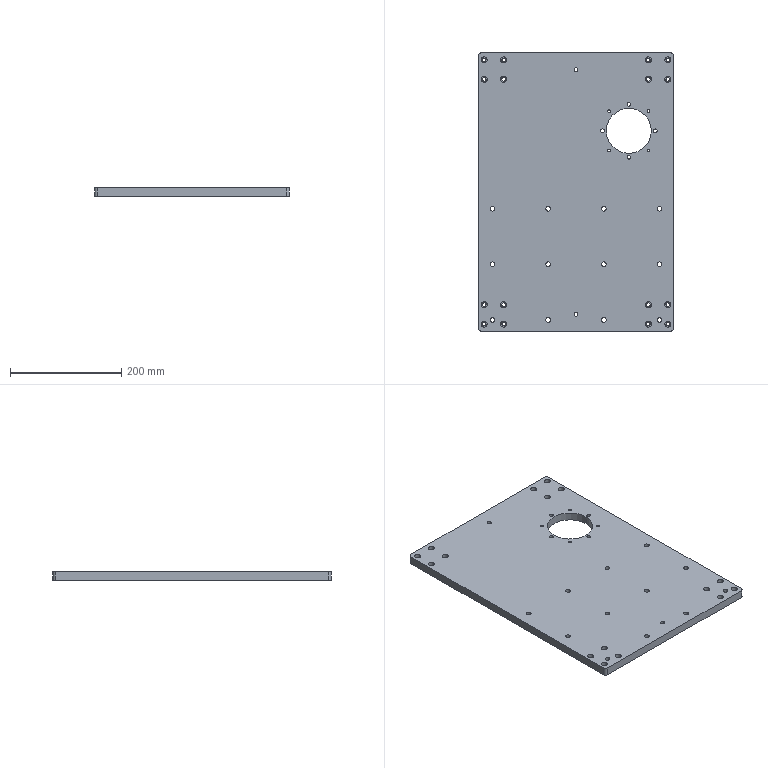NC program | Mastercam | posted with a generic post | part box 350 x 500 x 15 mm
Lines 1 to 1450 of 4195:
%
O0000()
(MATERIAL - ALUMINUM MM - 2024)
( T24 | 100 FEM | H24 )
( T9 | 10 FEM | H9 | XY STOCK TO LEAVE - .15 | Z STOCK TO LEAVE - .05 )
( T10 | 10 FEM | H10 | XY STOCK TO LEAVE - 0. | Z STOCK TO LEAVE - .05 )
( T7 | 4 CHM | H7 )
( T6 | 6 FEM | H6 )
N100 G21
N110 G0 G17 G40 G49 G80 G90
N120 T24 M6
N130 G0 G90 G54 X-360. Y144.998 A0. S4000 M3
N140 G43 H24 Z50. M8
N150 Z2.
N160 G1 Z0. F600.
N170 X300. F1000.
N180 G2 X336.249 Y108.749 I0. J-36.249
N190 X300. Y72.499 I-36.249 J0.
N200 G1 X-300.
N210 G3 X-336.25 Y36.249 I0. J-36.25
N220 X-300. Y0. I36.25 J0.
N230 G1 X300.
N240 G2 X336.249 Y-36.249 I0. J-36.249
N250 X300. Y-72.499 I-36.249 J0.
N260 G1 X-300.
N270 G3 X-336.25 Y-108.749 I0. J-36.25
N280 X-300. Y-144.998 I36.25 J0.
N290 G1 X360.
N300 G0 Z50.
N310 M5
N320 G91 G28 Z0. M9
N330 A0.
N340 M01
N350 T9 M6
N360 G0 G90 G17 G54 X-257.127 Y180.713 A0. S7000 M3
N370 G43 H9 Z50. M8
N380 Z1.
N390 G1 Z0. F600.
N400 X-253.591 Y177.177 F3000.
N410 G3 X-252.884 Y176.884 I.707 J.707
N420 X-252.177 Y177.177 I0. J1.
N430 G1 X-251.592 Y177.718
N440 X-250.966 Y178.211
N450 X-250.303 Y178.654 Z-.001
N460 X-249.608 Y179.044
N470 X-248.884 Y179.377
N480 X-248.136 Y179.653
N490 X-247.369 Y179.869
N500 X-246.588 Y180.025 Z-.002
N510 X-245.796 Y180.119
N520 X-245. Y180.15
N530 X245. Z-.144
N540 G2 X255.15 Y170. Z-.149 I0. J-10.15
N550 G1 Y-170. Z-.248
N560 X255.115 Y-170.838
N570 X255.012 Y-171.671
N580 X254.839 Y-172.492 Z-.249
N590 X254.6 Y-173.296
N600 X254.295 Y-174.077
N610 X253.927 Y-174.831
N620 X253.497 Y-175.552
N630 X253.01 Y-176.234 Z-.25
N640 X252.468 Y-176.874
N650 X251.874 Y-177.468
N660 X251.234 Y-178.01
N670 X250.552 Y-178.497 Z-.251
N680 X249.831 Y-178.927
N690 X249.077 Y-179.295
N700 X248.296 Y-179.6
N710 X247.492 Y-179.839
N720 X246.671 Y-180.012 Z-.252
N730 X245.838 Y-180.115
N740 X245. Y-180.15
N750 X-245. Z-.394
N760 G2 X-255.15 Y-170. Z-.399 I0. J10.15
N770 G1 Y170. Z-.498
N780 X-255.119 Y170.796
N790 X-255.025 Y171.588
N800 X-254.87 Y172.369 Z-.499
N810 X-254.653 Y173.137
N820 X-254.377 Y173.884
N830 X-254.044 Y174.608
N840 X-253.654 Y175.303
N850 X-253.212 Y175.966 Z-.5
N860 X-252.718 Y176.592
N870 X-252.177 Y177.177
N880 X-251.592 Y177.718
N890 X-250.966 Y178.211
N900 X-250.303 Y178.654 Z-.501
N910 X-249.608 Y179.044
N920 X-248.884 Y179.377
N930 X-248.136 Y179.653
N940 X-247.369 Y179.869
N950 X-246.588 Y180.025 Z-.502
N960 X-245.796 Y180.119
N970 X-245. Y180.15
N980 X245. Z-.644
N990 G2 X255.15 Y170. Z-.649 I0. J-10.15
N1000 G1 Y-170. Z-.748
N1010 X255.115 Y-170.838
N1020 X255.012 Y-171.671
N1030 X254.839 Y-172.492 Z-.749
N1040 X254.6 Y-173.296
N1050 X254.295 Y-174.077
N1060 X253.927 Y-174.831
N1070 X253.497 Y-175.552
N1080 X253.01 Y-176.234 Z-.75
N1090 X252.468 Y-176.874
N1100 X251.874 Y-177.468
N1110 X251.234 Y-178.01
N1120 X250.552 Y-178.497 Z-.751
N1130 X249.831 Y-178.927
N1140 X249.077 Y-179.295
N1150 X248.296 Y-179.6
N1160 X247.492 Y-179.839
N1170 X246.671 Y-180.012 Z-.752
N1180 X245.838 Y-180.115
N1190 X245. Y-180.15
N1200 X-245. Z-.894
N1210 G2 X-255.15 Y-170. Z-.899 I0. J10.15
N1220 G1 Y170. Z-.998
N1230 X-255.119 Y170.796
N1240 X-255.025 Y171.588
N1250 X-254.87 Y172.369 Z-.999
N1260 X-254.653 Y173.137
N1270 X-254.377 Y173.884
N1280 X-254.044 Y174.608
N1290 X-253.654 Y175.303
N1300 X-253.212 Y175.966 Z-1.
N1310 X-252.718 Y176.592
N1320 X-252.177 Y177.177
N1330 X-251.592 Y177.718
N1340 X-250.966 Y178.211
N1350 X-250.303 Y178.654 Z-1.001
N1360 X-249.608 Y179.044
N1370 X-248.884 Y179.377
N1380 X-248.136 Y179.653
N1390 X-247.369 Y179.869
N1400 X-246.588 Y180.025 Z-1.002
N1410 X-245.796 Y180.119
N1420 X-245. Y180.15
N1430 X245. Z-1.144
N1440 G2 X255.15 Y170. Z-1.149 I0. J-10.15
N1450 G1 Y-170. Z-1.248
N1460 X255.115 Y-170.838
N1470 X255.012 Y-171.671
N1480 X254.839 Y-172.492 Z-1.249
N1490 X254.6 Y-173.296
N1500 X254.295 Y-174.077
N1510 X253.927 Y-174.831
N1520 X253.497 Y-175.552
N1530 X253.01 Y-176.234 Z-1.25
N1540 X252.468 Y-176.874
N1550 X251.874 Y-177.468
N1560 X251.234 Y-178.01
N1570 X250.552 Y-178.497 Z-1.251
N1580 X249.831 Y-178.927
N1590 X249.077 Y-179.295
N1600 X248.296 Y-179.6
N1610 X247.492 Y-179.839
N1620 X246.671 Y-180.012 Z-1.252
N1630 X245.838 Y-180.115
N1640 X245. Y-180.15
N1650 X-245. Z-1.394
N1660 G2 X-255.15 Y-170. Z-1.399 I0. J10.15
N1670 G1 Y170. Z-1.498
N1680 X-255.119 Y170.796
N1690 X-255.025 Y171.588
N1700 X-254.87 Y172.369 Z-1.499
N1710 X-254.653 Y173.137
N1720 X-254.377 Y173.884
N1730 X-254.044 Y174.608
N1740 X-253.654 Y175.303
N1750 X-253.212 Y175.966 Z-1.5
N1760 X-252.718 Y176.592
N1770 X-252.177 Y177.177
N1780 X-251.592 Y177.718
N1790 X-250.966 Y178.211
N1800 X-250.303 Y178.654 Z-1.501
N1810 X-249.608 Y179.044
N1820 X-248.884 Y179.377
N1830 X-248.136 Y179.653
N1840 X-247.369 Y179.869
N1850 X-246.588 Y180.025 Z-1.502
N1860 X-245.796 Y180.119
N1870 X-245. Y180.15
N1880 X245. Z-1.644
N1890 G2 X255.15 Y170. Z-1.649 I0. J-10.15
N1900 G1 Y-170. Z-1.748
N1910 X255.115 Y-170.838
N1920 X255.012 Y-171.671
N1930 X254.839 Y-172.492 Z-1.749
N1940 X254.6 Y-173.296
N1950 X254.295 Y-174.077
N1960 X253.927 Y-174.831
N1970 X253.497 Y-175.552
N1980 X253.01 Y-176.234 Z-1.75
N1990 X252.468 Y-176.874
N2000 X251.874 Y-177.468
N2010 X251.234 Y-178.01
N2020 X250.552 Y-178.497 Z-1.751
N2030 X249.831 Y-178.927
N2040 X249.077 Y-179.295
N2050 X248.296 Y-179.6
N2060 X247.492 Y-179.839
N2070 X246.671 Y-180.012 Z-1.752
N2080 X245.838 Y-180.115
N2090 X245. Y-180.15
N2100 X-245. Z-1.894
N2110 G2 X-255.15 Y-170. Z-1.899 I0. J10.15
N2120 G1 Y170. Z-1.998
N2130 X-255.119 Y170.796
N2140 X-255.025 Y171.588
N2150 X-254.87 Y172.369 Z-1.999
N2160 X-254.653 Y173.137
N2170 X-254.377 Y173.884
N2180 X-254.044 Y174.608
N2190 X-253.654 Y175.303
N2200 X-253.212 Y175.966 Z-2.
N2210 X-252.718 Y176.592
N2220 X-252.177 Y177.177
N2230 X-251.592 Y177.718
N2240 X-250.966 Y178.211
N2250 X-250.303 Y178.654 Z-2.001
N2260 X-249.608 Y179.044
N2270 X-248.884 Y179.377
N2280 X-248.136 Y179.653
N2290 X-247.369 Y179.869
N2300 X-246.588 Y180.025 Z-2.002
N2310 X-245.796 Y180.119
N2320 X-245. Y180.15
N2330 X245. Z-2.144
N2340 G2 X255.15 Y170. Z-2.149 I0. J-10.15
N2350 G1 Y-170. Z-2.248
N2360 X255.115 Y-170.838
N2370 X255.012 Y-171.671
N2380 X254.839 Y-172.492 Z-2.249
N2390 X254.6 Y-173.296
N2400 X254.295 Y-174.077
N2410 X253.927 Y-174.831
N2420 X253.497 Y-175.552
N2430 X253.01 Y-176.234 Z-2.25
N2440 X252.468 Y-176.874
N2450 X251.874 Y-177.468
N2460 X251.234 Y-178.01
N2470 X250.552 Y-178.497 Z-2.251
N2480 X249.831 Y-178.927
N2490 X249.077 Y-179.295
N2500 X248.296 Y-179.6
N2510 X247.492 Y-179.839
N2520 X246.671 Y-180.012 Z-2.252
N2530 X245.838 Y-180.115
N2540 X245. Y-180.15
N2550 X-245. Z-2.394
N2560 G2 X-255.15 Y-170. Z-2.399 I0. J10.15
N2570 G1 Y170. Z-2.498
N2580 X-255.119 Y170.796
N2590 X-255.025 Y171.588
N2600 X-254.87 Y172.369 Z-2.499
N2610 X-254.653 Y173.137
N2620 X-254.377 Y173.884
N2630 X-254.044 Y174.608
N2640 X-253.654 Y175.303
N2650 X-253.212 Y175.966 Z-2.5
N2660 X-252.718 Y176.592
N2670 X-252.177 Y177.177
N2680 X-251.592 Y177.718
N2690 X-250.966 Y178.211
N2700 X-250.303 Y178.654 Z-2.501
N2710 X-249.608 Y179.044
N2720 X-248.884 Y179.377
N2730 X-248.136 Y179.653
N2740 X-247.369 Y179.869
N2750 X-246.588 Y180.025 Z-2.502
N2760 X-245.796 Y180.119
N2770 X-245. Y180.15
N2780 X245. Z-2.644
N2790 G2 X255.15 Y170. Z-2.649 I0. J-10.15
N2800 G1 Y-170. Z-2.748
N2810 X255.115 Y-170.838
N2820 X255.012 Y-171.671
N2830 X254.839 Y-172.492 Z-2.749
N2840 X254.6 Y-173.296
N2850 X254.295 Y-174.077
N2860 X253.927 Y-174.831
N2870 X253.497 Y-175.552
N2880 X253.01 Y-176.234 Z-2.75
N2890 X252.468 Y-176.874
N2900 X251.874 Y-177.468
N2910 X251.234 Y-178.01
N2920 X250.552 Y-178.497 Z-2.751
N2930 X249.831 Y-178.927
N2940 X249.077 Y-179.295
N2950 X248.296 Y-179.6
N2960 X247.492 Y-179.839
N2970 X246.671 Y-180.012 Z-2.752
N2980 X245.838 Y-180.115
N2990 X245. Y-180.15
N3000 X-245. Z-2.894
N3010 G2 X-255.15 Y-170. Z-2.899 I0. J10.15
N3020 G1 Y170. Z-2.998
N3030 X-255.119 Y170.796
N3040 X-255.025 Y171.588
N3050 X-254.87 Y172.369 Z-2.999
N3060 X-254.653 Y173.137
N3070 X-254.377 Y173.884
N3080 X-254.044 Y174.608
N3090 X-253.654 Y175.303
N3100 X-253.212 Y175.966 Z-3.
N3110 X-252.718 Y176.592
N3120 X-252.177 Y177.177
N3130 X-251.592 Y177.718
N3140 X-250.966 Y178.211
N3150 X-250.303 Y178.654 Z-3.001
N3160 X-249.608 Y179.044
N3170 X-248.884 Y179.377
N3180 X-248.136 Y179.653
N3190 X-247.369 Y179.869
N3200 X-246.588 Y180.025 Z-3.002
N3210 X-245.796 Y180.119
N3220 X-245. Y180.15
N3230 X245. Z-3.144
N3240 G2 X255.15 Y170. Z-3.149 I0. J-10.15
N3250 G1 Y-170. Z-3.248
N3260 X255.115 Y-170.838
N3270 X255.012 Y-171.671
N3280 X254.839 Y-172.492 Z-3.249
N3290 X254.6 Y-173.296
N3300 X254.295 Y-174.077
N3310 X253.927 Y-174.831
N3320 X253.497 Y-175.552
N3330 X253.01 Y-176.234 Z-3.25
N3340 X252.468 Y-176.874
N3350 X251.874 Y-177.468
N3360 X251.234 Y-178.01
N3370 X250.552 Y-178.497 Z-3.251
N3380 X249.831 Y-178.927
N3390 X249.077 Y-179.295
N3400 X248.296 Y-179.6
N3410 X247.492 Y-179.839
N3420 X246.671 Y-180.012 Z-3.252
N3430 X245.838 Y-180.115
N3440 X245. Y-180.15
N3450 X-245. Z-3.394
N3460 G2 X-255.15 Y-170. Z-3.399 I0. J10.15
N3470 G1 Y170. Z-3.498
N3480 X-255.119 Y170.796
N3490 X-255.025 Y171.588
N3500 X-254.87 Y172.369 Z-3.499
N3510 X-254.653 Y173.137
N3520 X-254.377 Y173.884
N3530 X-254.044 Y174.608
N3540 X-253.654 Y175.303
N3550 X-253.212 Y175.966 Z-3.5
N3560 X-252.718 Y176.592
N3570 X-252.177 Y177.177
N3580 X-251.592 Y177.718
N3590 X-250.966 Y178.211
N3600 X-250.303 Y178.654 Z-3.501
N3610 X-249.608 Y179.044
N3620 X-248.884 Y179.377
N3630 X-248.136 Y179.653
N3640 X-247.369 Y179.869
N3650 X-246.588 Y180.025 Z-3.502
N3660 X-245.796 Y180.119
N3670 X-245. Y180.15
N3680 X245. Z-3.644
N3690 G2 X255.15 Y170. Z-3.649 I0. J-10.15
N3700 G1 Y-170. Z-3.748
N3710 X255.115 Y-170.838
N3720 X255.012 Y-171.671
N3730 X254.839 Y-172.492 Z-3.749
N3740 X254.6 Y-173.296
N3750 X254.295 Y-174.077
N3760 X253.927 Y-174.831
N3770 X253.497 Y-175.552
N3780 X253.01 Y-176.234 Z-3.75
N3790 X252.468 Y-176.874
N3800 X251.874 Y-177.468
N3810 X251.234 Y-178.01
N3820 X250.552 Y-178.497 Z-3.751
N3830 X249.831 Y-178.927
N3840 X249.077 Y-179.295
N3850 X248.296 Y-179.6
N3860 X247.492 Y-179.839
N3870 X246.671 Y-180.012 Z-3.752
N3880 X245.838 Y-180.115
N3890 X245. Y-180.15
N3900 X-245. Z-3.894
N3910 G2 X-255.15 Y-170. Z-3.899 I0. J10.15
N3920 G1 Y170. Z-3.998
N3930 X-255.119 Y170.796
N3940 X-255.025 Y171.588
N3950 X-254.87 Y172.369 Z-3.999
N3960 X-254.653 Y173.137
N3970 X-254.377 Y173.884
N3980 X-254.044 Y174.608
N3990 X-253.654 Y175.303
N4000 X-253.212 Y175.966 Z-4.
N4010 X-252.718 Y176.592
N4020 X-252.177 Y177.177
N4030 X-251.592 Y177.718
N4040 X-250.966 Y178.211
N4050 X-250.303 Y178.654 Z-4.001
N4060 X-249.608 Y179.044
N4070 X-248.884 Y179.377
N4080 X-248.136 Y179.653
N4090 X-247.369 Y179.869
N4100 X-246.588 Y180.025 Z-4.002
N4110 X-245.796 Y180.119
N4120 X-245. Y180.15
N4130 X245. Z-4.144
N4140 G2 X255.15 Y170. Z-4.149 I0. J-10.15
N4150 G1 Y-170. Z-4.248
N4160 X255.115 Y-170.838
N4170 X255.012 Y-171.671
N4180 X254.839 Y-172.492 Z-4.249
N4190 X254.6 Y-173.296
N4200 X254.295 Y-174.077
N4210 X253.927 Y-174.831
N4220 X253.497 Y-175.552
N4230 X253.01 Y-176.234 Z-4.25
N4240 X252.468 Y-176.874
N4250 X251.874 Y-177.468
N4260 X251.234 Y-178.01
N4270 X250.552 Y-178.497 Z-4.251
N4280 X249.831 Y-178.927
N4290 X249.077 Y-179.295
N4300 X248.296 Y-179.6
N4310 X247.492 Y-179.839
N4320 X246.671 Y-180.012 Z-4.252
N4330 X245.838 Y-180.115
N4340 X245. Y-180.15
N4350 X-245. Z-4.394
N4360 G2 X-255.15 Y-170. Z-4.399 I0. J10.15
N4370 G1 Y170. Z-4.498
N4380 X-255.119 Y170.796
N4390 X-255.025 Y171.588
N4400 X-254.87 Y172.369 Z-4.499
N4410 X-254.653 Y173.137
N4420 X-254.377 Y173.884
N4430 X-254.044 Y174.608
N4440 X-253.654 Y175.303
N4450 X-253.212 Y175.966 Z-4.5
N4460 X-252.718 Y176.592
N4470 X-252.177 Y177.177
N4480 X-251.592 Y177.718
N4490 X-250.966 Y178.211
N4500 X-250.303 Y178.654 Z-4.501
N4510 X-249.608 Y179.044
N4520 X-248.884 Y179.377
N4530 X-248.136 Y179.653
N4540 X-247.369 Y179.869
N4550 X-246.588 Y180.025 Z-4.502
N4560 X-245.796 Y180.119
N4570 X-245. Y180.15
N4580 X245. Z-4.644
N4590 G2 X255.15 Y170. Z-4.649 I0. J-10.15
N4600 G1 Y-170. Z-4.748
N4610 X255.115 Y-170.838
N4620 X255.012 Y-171.671
N4630 X254.839 Y-172.492 Z-4.749
N4640 X254.6 Y-173.296
N4650 X254.295 Y-174.077
N4660 X253.927 Y-174.831
N4670 X253.497 Y-175.552
N4680 X253.01 Y-176.234 Z-4.75
N4690 X252.468 Y-176.874
N4700 X251.874 Y-177.468
N4710 X251.234 Y-178.01
N4720 X250.552 Y-178.497 Z-4.751
N4730 X249.831 Y-178.927
N4740 X249.077 Y-179.295
N4750 X248.296 Y-179.6
N4760 X247.492 Y-179.839
N4770 X246.671 Y-180.012 Z-4.752
N4780 X245.838 Y-180.115
N4790 X245. Y-180.15
N4800 X-245. Z-4.894
N4810 G2 X-255.15 Y-170. Z-4.899 I0. J10.15
N4820 G1 Y170. Z-4.998
N4830 X-255.119 Y170.796
N4840 X-255.025 Y171.588
N4850 X-254.87 Y172.369 Z-4.999
N4860 X-254.653 Y173.137
N4870 X-254.377 Y173.884
N4880 X-254.044 Y174.608
N4890 X-253.654 Y175.303
N4900 X-253.212 Y175.966 Z-5.
N4910 X-252.718 Y176.592
N4920 X-252.177 Y177.177
N4930 X-251.592 Y177.718
N4940 X-250.966 Y178.211
N4950 X-250.303 Y178.654 Z-5.001
N4960 X-249.608 Y179.044
N4970 X-248.884 Y179.377
N4980 X-248.136 Y179.653
N4990 X-247.369 Y179.869
N5000 X-246.588 Y180.025 Z-5.002
N5010 X-245.796 Y180.119
N5020 X-245. Y180.15
N5030 X245. Z-5.144
N5040 G2 X255.15 Y170. Z-5.149 I0. J-10.15
N5050 G1 Y-170. Z-5.248
N5060 X255.115 Y-170.838
N5070 X255.012 Y-171.671
N5080 X254.839 Y-172.492 Z-5.249
N5090 X254.6 Y-173.296
N5100 X254.295 Y-174.077
N5110 X253.927 Y-174.831
N5120 X253.497 Y-175.552
N5130 X253.01 Y-176.234 Z-5.25
N5140 X252.468 Y-176.874
N5150 X251.874 Y-177.468
N5160 X251.234 Y-178.01
N5170 X250.552 Y-178.497 Z-5.251
N5180 X249.831 Y-178.927
N5190 X249.077 Y-179.295
N5200 X248.296 Y-179.6
N5210 X247.492 Y-179.839
N5220 X246.671 Y-180.012 Z-5.252
N5230 X245.838 Y-180.115
N5240 X245. Y-180.15
N5250 X-245. Z-5.394
N5260 G2 X-255.15 Y-170. Z-5.399 I0. J10.15
N5270 G1 Y170. Z-5.498
N5280 X-255.119 Y170.796
N5290 X-255.025 Y171.588
N5300 X-254.87 Y172.369 Z-5.499
N5310 X-254.653 Y173.137
N5320 X-254.377 Y173.884
N5330 X-254.044 Y174.608
N5340 X-253.654 Y175.303
N5350 X-253.212 Y175.966 Z-5.5
N5360 X-252.718 Y176.592
N5370 X-252.177 Y177.177
N5380 X-251.592 Y177.718
N5390 X-250.966 Y178.211
N5400 X-250.303 Y178.654 Z-5.501
N5410 X-249.608 Y179.044
N5420 X-248.884 Y179.377
N5430 X-248.136 Y179.653
N5440 X-247.369 Y179.869
N5450 X-246.588 Y180.025 Z-5.502
N5460 X-245.796 Y180.119
N5470 X-245. Y180.15
N5480 X245. Z-5.644
N5490 G2 X255.15 Y170. Z-5.649 I0. J-10.15
N5500 G1 Y-170. Z-5.748
N5510 X255.115 Y-170.838
N5520 X255.012 Y-171.671
N5530 X254.839 Y-172.492 Z-5.749
N5540 X254.6 Y-173.296
N5550 X254.295 Y-174.077
N5560 X253.927 Y-174.831
N5570 X253.497 Y-175.552
N5580 X253.01 Y-176.234 Z-5.75
N5590 X252.468 Y-176.874
N5600 X251.874 Y-177.468
N5610 X251.234 Y-178.01
N5620 X250.552 Y-178.497 Z-5.751
N5630 X249.831 Y-178.927
N5640 X249.077 Y-179.295
N5650 X248.296 Y-179.6
N5660 X247.492 Y-179.839
N5670 X246.671 Y-180.012 Z-5.752
N5680 X245.838 Y-180.115
N5690 X245. Y-180.15
N5700 X-245. Z-5.894
N5710 G2 X-255.15 Y-170. Z-5.899 I0. J10.15
N5720 G1 Y170. Z-5.998
N5730 X-255.119 Y170.796
N5740 X-255.025 Y171.588
N5750 X-254.87 Y172.369 Z-5.999
N5760 X-254.653 Y173.137
N5770 X-254.377 Y173.884
N5780 X-254.044 Y174.608
N5790 X-253.654 Y175.303
N5800 X-253.212 Y175.966 Z-6.
N5810 X-252.718 Y176.592
N5820 X-252.177 Y177.177
N5830 X-251.592 Y177.718
N5840 X-250.966 Y178.211
N5850 X-250.303 Y178.654 Z-6.001
N5860 X-249.608 Y179.044
N5870 X-248.884 Y179.377
N5880 X-248.136 Y179.653
N5890 X-247.369 Y179.869
N5900 X-246.588 Y180.025 Z-6.002
N5910 X-245.796 Y180.119
N5920 X-245. Y180.15
N5930 X245. Z-6.144
N5940 G2 X255.15 Y170. Z-6.149 I0. J-10.15
N5950 G1 Y-170. Z-6.248
N5960 X255.115 Y-170.838
N5970 X255.012 Y-171.671
N5980 X254.839 Y-172.492 Z-6.249
N5990 X254.6 Y-173.296
N6000 X254.295 Y-174.077
N6010 X253.927 Y-174.831
N6020 X253.497 Y-175.552
N6030 X253.01 Y-176.234 Z-6.25
N6040 X252.468 Y-176.874
N6050 X251.874 Y-177.468
N6060 X251.234 Y-178.01
N6070 X250.552 Y-178.497 Z-6.251
N6080 X249.831 Y-178.927
N6090 X249.077 Y-179.295
N6100 X248.296 Y-179.6
N6110 X247.492 Y-179.839
N6120 X246.671 Y-180.012 Z-6.252
N6130 X245.838 Y-180.115
N6140 X245. Y-180.15
N6150 X-245. Z-6.394
N6160 G2 X-255.15 Y-170. Z-6.399 I0. J10.15
N6170 G1 Y170. Z-6.498
N6180 X-255.119 Y170.796
N6190 X-255.025 Y171.588
N6200 X-254.87 Y172.369 Z-6.499
N6210 X-254.653 Y173.137
N6220 X-254.377 Y173.884
N6230 X-254.044 Y174.608
N6240 X-253.654 Y175.303
N6250 X-253.212 Y175.966 Z-6.5
N6260 X-252.718 Y176.592
N6270 X-252.177 Y177.177
N6280 X-251.592 Y177.718
N6290 X-250.966 Y178.211
N6300 X-250.303 Y178.654 Z-6.501
N6310 X-249.608 Y179.044
N6320 X-248.884 Y179.377
N6330 X-248.136 Y179.653
N6340 X-247.369 Y179.869
N6350 X-246.588 Y180.025 Z-6.502
N6360 X-245.796 Y180.119
N6370 X-245. Y180.15
N6380 X245. Z-6.644
N6390 G2 X255.15 Y170. Z-6.649 I0. J-10.15
N6400 G1 Y-170. Z-6.748
N6410 X255.115 Y-170.838
N6420 X255.012 Y-171.671
N6430 X254.839 Y-172.492 Z-6.749
N6440 X254.6 Y-173.296
N6450 X254.295 Y-174.077
N6460 X253.927 Y-174.831
N6470 X253.497 Y-175.552
N6480 X253.01 Y-176.234 Z-6.75
N6490 X252.468 Y-176.874
N6500 X251.874 Y-177.468
N6510 X251.234 Y-178.01
N6520 X250.552 Y-178.497 Z-6.751
N6530 X249.831 Y-178.927
N6540 X249.077 Y-179.295
N6550 X248.296 Y-179.6
N6560 X247.492 Y-179.839
N6570 X246.671 Y-180.012 Z-6.752
N6580 X245.838 Y-180.115
N6590 X245. Y-180.15
N6600 X-245. Z-6.894
N6610 G2 X-255.15 Y-170. Z-6.899 I0. J10.15
N6620 G1 Y170. Z-6.998
N6630 X-255.119 Y170.796
N6640 X-255.025 Y171.588
N6650 X-254.87 Y172.369 Z-6.999
N6660 X-254.653 Y173.137
N6670 X-254.377 Y173.884
N6680 X-254.044 Y174.608
N6690 X-253.654 Y175.303
N6700 X-253.212 Y175.966 Z-7.
N6710 X-252.718 Y176.592
N6720 X-252.177 Y177.177
N6730 X-251.592 Y177.718
N6740 X-250.966 Y178.211
N6750 X-250.303 Y178.654 Z-7.001
N6760 X-249.608 Y179.044
N6770 X-248.884 Y179.377
N6780 X-248.136 Y179.653
N6790 X-247.369 Y179.869
N6800 X-246.588 Y180.025 Z-7.002
N6810 X-245.796 Y180.119
N6820 X-245. Y180.15
N6830 X245. Z-7.144
N6840 G2 X255.15 Y170. Z-7.149 I0. J-10.15
N6850 G1 Y-170. Z-7.248
N6860 X255.115 Y-170.838
N6870 X255.012 Y-171.671
N6880 X254.839 Y-172.492 Z-7.249
N6890 X254.6 Y-173.296
N6900 X254.295 Y-174.077
N6910 X253.927 Y-174.831
N6920 X253.497 Y-175.552
N6930 X253.01 Y-176.234 Z-7.25
N6940 X252.468 Y-176.874
N6950 X251.874 Y-177.468
N6960 X251.234 Y-178.01
N6970 X250.552 Y-178.497 Z-7.251
N6980 X249.831 Y-178.927
N6990 X249.077 Y-179.295
N7000 X248.296 Y-179.6
N7010 X247.492 Y-179.839
N7020 X246.671 Y-180.012 Z-7.252
N7030 X245.838 Y-180.115
N7040 X245. Y-180.15
N7050 X-245. Z-7.394
N7060 G2 X-255.15 Y-170. Z-7.399 I0. J10.15
N7070 G1 Y170. Z-7.498
N7080 X-255.119 Y170.796
N7090 X-255.025 Y171.588
N7100 X-254.87 Y172.369 Z-7.499
N7110 X-254.653 Y173.137
N7120 X-254.377 Y173.884
N7130 X-254.044 Y174.608
N7140 X-253.654 Y175.303
N7150 X-253.212 Y175.966 Z-7.5
N7160 X-252.718 Y176.592
N7170 X-252.177 Y177.177
N7180 X-251.592 Y177.718
N7190 X-250.966 Y178.211
N7200 X-250.303 Y178.654 Z-7.501
N7210 X-249.608 Y179.044
N7220 X-248.884 Y179.377
N7230 X-248.136 Y179.653
N7240 X-247.369 Y179.869
N7250 X-246.588 Y180.025 Z-7.502
N7260 X-245.796 Y180.119
N7270 X-245. Y180.15
N7280 X245. Z-7.644
N7290 G2 X255.15 Y170. Z-7.649 I0. J-10.15
N7300 G1 Y-170. Z-7.748
N7310 X255.115 Y-170.838
N7320 X255.012 Y-171.671
N7330 X254.839 Y-172.492 Z-7.749
N7340 X254.6 Y-173.296
N7350 X254.295 Y-174.077
N7360 X253.927 Y-174.831
N7370 X253.497 Y-175.552
N7380 X253.01 Y-176.234 Z-7.75
N7390 X252.468 Y-176.874
N7400 X251.874 Y-177.468
N7410 X251.234 Y-178.01
N7420 X250.552 Y-178.497 Z-7.751
N7430 X249.831 Y-178.927
N7440 X249.077 Y-179.295
N7450 X248.296 Y-179.6
N7460 X247.492 Y-179.839
N7470 X246.671 Y-180.012 Z-7.752
N7480 X245.838 Y-180.115
N7490 X245. Y-180.15
N7500 X-245. Z-7.894
N7510 G2 X-255.15 Y-170. Z-7.899 I0. J10.15
N7520 G1 Y170. Z-7.998
N7530 X-255.119 Y170.796
N7540 X-255.025 Y171.588
N7550 X-254.87 Y172.369 Z-7.999
N7560 X-254.653 Y173.137
N7570 X-254.377 Y173.884
N7580 X-254.044 Y174.608
N7590 X-253.654 Y175.303
N7600 X-253.212 Y175.966 Z-8.
N7610 X-252.718 Y176.592
N7620 X-252.177 Y177.177
N7630 X-251.592 Y177.718
N7640 X-250.966 Y178.211
N7650 X-250.303 Y178.654 Z-8.001
N7660 X-249.608 Y179.044
N7670 X-248.884 Y179.377
N7680 X-248.136 Y179.653
N7690 X-247.369 Y179.869
N7700 X-246.588 Y180.025 Z-8.002
N7710 X-245.796 Y180.119
N7720 X-245. Y180.15
N7730 X245. Z-8.144
N7740 G2 X255.15 Y170. Z-8.149 I0. J-10.15
N7750 G1 Y-170. Z-8.248
N7760 X255.115 Y-170.838
N7770 X255.012 Y-171.671
N7780 X254.839 Y-172.492 Z-8.249
N7790 X254.6 Y-173.296
N7800 X254.295 Y-174.077
N7810 X253.927 Y-174.831
N7820 X253.497 Y-175.552
N7830 X253.01 Y-176.234 Z-8.25
N7840 X252.468 Y-176.874
N7850 X251.874 Y-177.468
N7860 X251.234 Y-178.01
N7870 X250.552 Y-178.497 Z-8.251
N7880 X249.831 Y-178.927
N7890 X249.077 Y-179.295
N7900 X248.296 Y-179.6
N7910 X247.492 Y-179.839
N7920 X246.671 Y-180.012 Z-8.252
N7930 X245.838 Y-180.115
N7940 X245. Y-180.15
N7950 X-245. Z-8.394
N7960 G2 X-255.15 Y-170. Z-8.399 I0. J10.15
N7970 G1 Y170. Z-8.498
N7980 X-255.119 Y170.796
N7990 X-255.025 Y171.588
N8000 X-254.87 Y172.369 Z-8.499
N8010 X-254.653 Y173.137
N8020 X-254.377 Y173.884
N8030 X-254.044 Y174.608
N8040 X-253.654 Y175.303
N8050 X-253.212 Y175.966 Z-8.5
N8060 X-252.718 Y176.592
N8070 X-252.177 Y177.177
N8080 X-251.592 Y177.718
N8090 X-250.966 Y178.211
N8100 X-250.303 Y178.654 Z-8.501
N8110 X-249.608 Y179.044
N8120 X-248.884 Y179.377
N8130 X-248.136 Y179.653
N8140 X-247.369 Y179.869
N8150 X-246.588 Y180.025 Z-8.502
N8160 X-245.796 Y180.119
N8170 X-245. Y180.15
N8180 X245. Z-8.644
N8190 G2 X255.15 Y170. Z-8.649 I0. J-10.15
N8200 G1 Y-170. Z-8.748
N8210 X255.115 Y-170.838
N8220 X255.012 Y-171.671
N8230 X254.839 Y-172.492 Z-8.749
N8240 X254.6 Y-173.296
N8250 X254.295 Y-174.077
N8260 X253.927 Y-174.831
N8270 X253.497 Y-175.552
N8280 X253.01 Y-176.234 Z-8.75
N8290 X252.468 Y-176.874
N8300 X251.874 Y-177.468
N8310 X251.234 Y-178.01
N8320 X250.552 Y-178.497 Z-8.751
N8330 X249.831 Y-178.927
N8340 X249.077 Y-179.295
N8350 X248.296 Y-179.6
N8360 X247.492 Y-179.839
N8370 X246.671 Y-180.012 Z-8.752
N8380 X245.838 Y-180.115
N8390 X245. Y-180.15
N8400 X-245. Z-8.894
N8410 G2 X-255.15 Y-170. Z-8.899 I0. J10.15
N8420 G1 Y170. Z-8.998
N8430 X-255.119 Y170.796
N8440 X-255.025 Y171.588
N8450 X-254.87 Y172.369 Z-8.999
N8460 X-254.653 Y173.137
N8470 X-254.377 Y173.884
N8480 X-254.044 Y174.608
N8490 X-253.654 Y175.303
N8500 X-253.212 Y175.966 Z-9.
N8510 X-252.718 Y176.592
N8520 X-252.177 Y177.177
N8530 X-251.592 Y177.718
N8540 X-250.966 Y178.211
N8550 X-250.303 Y178.654 Z-9.001
N8560 X-249.608 Y179.044
N8570 X-248.884 Y179.377
N8580 X-248.136 Y179.653
N8590 X-247.369 Y179.869
N8600 X-246.588 Y180.025 Z-9.002
N8610 X-245.796 Y180.119
N8620 X-245. Y180.15
N8630 X245. Z-9.144
N8640 G2 X255.15 Y170. Z-9.149 I0. J-10.15
N8650 G1 Y-170. Z-9.248
N8660 X255.115 Y-170.838
N8670 X255.012 Y-171.671
N8680 X254.839 Y-172.492 Z-9.249
N8690 X254.6 Y-173.296
N8700 X254.295 Y-174.077
N8710 X253.927 Y-174.831
N8720 X253.497 Y-175.552
N8730 X253.01 Y-176.234 Z-9.25
N8740 X252.468 Y-176.874
N8750 X251.874 Y-177.468
N8760 X251.234 Y-178.01
N8770 X250.552 Y-178.497 Z-9.251
N8780 X249.831 Y-178.927
N8790 X249.077 Y-179.295
N8800 X248.296 Y-179.6
N8810 X247.492 Y-179.839
N8820 X246.671 Y-180.012 Z-9.252
N8830 X245.838 Y-180.115
N8840 X245. Y-180.15
N8850 X-245. Z-9.394
N8860 G2 X-255.15 Y-170. Z-9.399 I0. J10.15
N8870 G1 Y170. Z-9.498
N8880 X-255.119 Y170.796
N8890 X-255.025 Y171.588
N8900 X-254.87 Y172.369 Z-9.499
N8910 X-254.653 Y173.137
N8920 X-254.377 Y173.884
N8930 X-254.044 Y174.608
N8940 X-253.654 Y175.303
N8950 X-253.212 Y175.966 Z-9.5
N8960 X-252.718 Y176.592
N8970 X-252.177 Y177.177
N8980 X-251.592 Y177.718
N8990 X-250.966 Y178.211
N9000 X-250.303 Y178.654 Z-9.501
N9010 X-249.608 Y179.044
N9020 X-248.884 Y179.377
N9030 X-248.136 Y179.653
N9040 X-247.369 Y179.869
N9050 X-246.588 Y180.025 Z-9.502
N9060 X-245.796 Y180.119
N9070 X-245. Y180.15
N9080 X245. Z-9.644
N9090 G2 X255.15 Y170. Z-9.649 I0. J-10.15
N9100 G1 Y-170. Z-9.748
N9110 X255.115 Y-170.838
N9120 X255.012 Y-171.671
N9130 X254.839 Y-172.492 Z-9.749
N9140 X254.6 Y-173.296
N9150 X254.295 Y-174.077
N9160 X253.927 Y-174.831
N9170 X253.497 Y-175.552
N9180 X253.01 Y-176.234 Z-9.75
N9190 X252.468 Y-176.874
N9200 X251.874 Y-177.468
N9210 X251.234 Y-178.01
N9220 X250.552 Y-178.497 Z-9.751
N9230 X249.831 Y-178.927
N9240 X249.077 Y-179.295
N9250 X248.296 Y-179.6
N9260 X247.492 Y-179.839
N9270 X246.671 Y-180.012 Z-9.752
N9280 X245.838 Y-180.115
N9290 X245. Y-180.15
N9300 X-245. Z-9.894
N9310 G2 X-255.15 Y-170. Z-9.899 I0. J10.15
N9320 G1 Y170. Z-9.998
N9330 X-255.119 Y170.796
N9340 X-255.025 Y171.588
N9350 X-254.87 Y172.369 Z-9.999
N9360 X-254.653 Y173.137
N9370 X-254.377 Y173.884
N9380 X-254.044 Y174.608
N9390 X-253.654 Y175.303
N9400 X-253.212 Y175.966 Z-10.
N9410 X-252.718 Y176.592
N9420 X-252.177 Y177.177
N9430 X-251.592 Y177.718
N9440 X-250.966 Y178.211
N9450 X-250.303 Y178.654 Z-10.001
N9460 X-249.608 Y179.044
N9470 X-248.884 Y179.377
N9480 X-248.136 Y179.653
N9490 X-247.369 Y179.869
N9500 X-246.588 Y180.025 Z-10.002
N9510 X-245.796 Y180.119
N9520 X-245. Y180.15
N9530 X245. Z-10.144
N9540 G2 X255.15 Y170. Z-10.149 I0. J-10.15
N9550 G1 Y-170. Z-10.248
N9560 X255.115 Y-170.838
N9570 X255.012 Y-171.671
N9580 X254.839 Y-172.492 Z-10.249
N9590 X254.6 Y-173.296
N9600 X254.295 Y-174.077
N9610 X253.927 Y-174.831
N9620 X253.497 Y-175.552
N9630 X253.01 Y-176.234 Z-10.25
N9640 X252.468 Y-176.874
N9650 X251.874 Y-177.468
N9660 X251.234 Y-178.01
N9670 X250.552 Y-178.497 Z-10.251
N9680 X249.831 Y-178.927
N9690 X249.077 Y-179.295
N9700 X248.296 Y-179.6
N9710 X247.492 Y-179.839
N9720 X246.671 Y-180.012 Z-10.252
N9730 X245.838 Y-180.115
N9740 X245. Y-180.15
N9750 X-245. Z-10.394
N9760 G2 X-255.15 Y-170. Z-10.399 I0. J10.15
N9770 G1 Y170. Z-10.498
N9780 X-255.119 Y170.796
N9790 X-255.025 Y171.588
N9800 X-254.87 Y172.369 Z-10.499
N9810 X-254.653 Y173.137
N9820 X-254.377 Y173.884
N9830 X-254.044 Y174.608
N9840 X-253.654 Y175.303
N9850 X-253.212 Y175.966 Z-10.5
N9860 X-252.718 Y176.592
N9870 X-252.177 Y177.177
N9880 X-251.592 Y177.718
N9890 X-250.966 Y178.211
N9900 X-250.303 Y178.654 Z-10.501
N9910 X-249.608 Y179.044
N9920 X-248.884 Y179.377
N9930 X-248.136 Y179.653
N9940 X-247.369 Y179.869
N9950 X-246.588 Y180.025 Z-10.502
N9960 X-245.796 Y180.119
N9970 X-245. Y180.15
N9980 X245. Z-10.644
N9990 G2 X255.15 Y170. Z-10.649 I0. J-10.15
N100 G1 Y-170. Z-10.748
N110 X255.115 Y-170.838
N120 X255.012 Y-171.671
N130 X254.839 Y-172.492 Z-10.749
N140 X254.6 Y-173.296
N150 X254.295 Y-174.077
N160 X253.927 Y-174.831
N170 X253.497 Y-175.552
N180 X253.01 Y-176.234 Z-10.75
N190 X252.468 Y-176.874
N200 X251.874 Y-177.468
N210 X251.234 Y-178.01
N220 X250.552 Y-178.497 Z-10.751
N230 X249.831 Y-178.927
N240 X249.077 Y-179.295
N250 X248.296 Y-179.6
N260 X247.492 Y-179.839
N270 X246.671 Y-180.012 Z-10.752
N280 X245.838 Y-180.115
N290 X245. Y-180.15
N300 X-245. Z-10.894
N310 G2 X-255.15 Y-170. Z-10.899 I0. J10.15
N320 G1 Y170. Z-10.998
N330 X-255.119 Y170.796
N340 X-255.025 Y171.588
N350 X-254.87 Y172.369 Z-10.999
N360 X-254.653 Y173.137
N370 X-254.377 Y173.884
N380 X-254.044 Y174.608
N390 X-253.654 Y175.303
N400 X-253.212 Y175.966 Z-11.
N410 X-252.718 Y176.592
N420 X-252.177 Y177.177
N430 X-251.592 Y177.718
N440 X-250.966 Y178.211
N450 X-250.303 Y178.654 Z-11.001
N460 X-249.608 Y179.044
N470 X-248.884 Y179.377
N480 X-248.136 Y179.653
N490 X-247.369 Y179.869
N500 X-246.588 Y180.025 Z-11.002
N510 X-245.796 Y180.119
N520 X-245. Y180.15
N530 X245. Z-11.144
N540 G2 X255.15 Y170. Z-11.149 I0. J-10.15
N550 G1 Y-170. Z-11.248
N560 X255.115 Y-170.838
N570 X255.012 Y-171.671
N580 X254.839 Y-172.492 Z-11.249
N590 X254.6 Y-173.296
N600 X254.295 Y-174.077
N610 X253.927 Y-174.831
N620 X253.497 Y-175.552
N630 X253.01 Y-176.234 Z-11.25
N640 X252.468 Y-176.874
N650 X251.874 Y-177.468
N660 X251.234 Y-178.01
N670 X250.552 Y-178.497 Z-11.251
N680 X249.831 Y-178.927
N690 X249.077 Y-179.295
N700 X248.296 Y-179.6
N710 X247.492 Y-179.839
N720 X246.671 Y-180.012 Z-11.252
N730 X245.838 Y-180.115
N740 X245. Y-180.15
N750 X-245. Z-11.394
N760 G2 X-255.15 Y-170. Z-11.399 I0. J10.15
N770 G1 Y170. Z-11.498
N780 X-255.119 Y170.796
N790 X-255.025 Y171.588
N800 X-254.87 Y172.369 Z-11.499
N810 X-254.653 Y173.137
N820 X-254.377 Y173.884
N830 X-254.044 Y174.608
N840 X-253.654 Y175.303
N850 X-253.212 Y175.966 Z-11.5
N860 X-252.718 Y176.592
N870 X-252.177 Y177.177
N880 X-251.592 Y177.718
N890 X-250.966 Y178.211
N900 X-250.303 Y178.654 Z-11.501
N910 X-249.608 Y179.044
N920 X-248.884 Y179.377
N930 X-248.136 Y179.653
N940 X-247.369 Y179.869
N950 X-246.588 Y180.025 Z-11.502
N960 X-245.796 Y180.119
N970 X-245. Y180.15
N980 X245. Z-11.644
N990 G2 X255.15 Y170. Z-11.649 I0. J-10.15
N1000 G1 Y-170. Z-11.748
N1010 X255.115 Y-170.838
N1020 X255.012 Y-171.671
N1030 X254.839 Y-172.492 Z-11.749
N1040 X254.6 Y-173.296
N1050 X254.295 Y-174.077
N1060 X253.927 Y-174.831
N1070 X253.497 Y-175.552
N1080 X253.01 Y-176.234 Z-11.75
N1090 X252.468 Y-176.874
N1100 X251.874 Y-177.468
N1110 X251.234 Y-178.01
N1120 X250.552 Y-178.497 Z-11.751
N1130 X249.831 Y-178.927
N1140 X249.077 Y-179.295
N1150 X248.296 Y-179.6
N1160 X247.492 Y-179.839
N1170 X246.671 Y-180.012 Z-11.752
N1180 X245.838 Y-180.115
N1190 X245. Y-180.15
N1200 X-245. Z-11.894
N1210 G2 X-255.15 Y-170. Z-11.899 I0. J10.15
N1220 G1 Y170. Z-11.998
N1230 X-255.119 Y170.796
N1240 X-255.025 Y171.588
N1250 X-254.87 Y172.369 Z-11.999
N1260 X-254.653 Y173.137
N1270 X-254.377 Y173.884
N1280 X-254.044 Y174.608
N1290 X-253.654 Y175.303
N1300 X-253.212 Y175.966 Z-12.
N1310 X-252.718 Y176.592
N1320 X-252.177 Y177.177
N1330 X-251.592 Y177.718
N1340 X-250.966 Y178.211
N1350 X-250.303 Y178.654 Z-12.001
N1360 X-249.608 Y179.044
N1370 X-248.884 Y179.377
N1380 X-248.136 Y179.653
N1390 X-247.369 Y179.869
N1400 X-246.588 Y180.025 Z-12.002
N1410 X-245.796 Y180.119
N1420 X-245. Y180.15
N1430 X245. Z-12.144
N1440 G2 X255.15 Y170. Z-12.149 I0. J-10.15
N1450 G1 Y-170. Z-12.248
N1460 X255.115 Y-170.838
N1470 X255.012 Y-171.671
N1480 X254.839 Y-172.492 Z-12.249
N1490 X254.6 Y-173.296
N1500 X254.295 Y-174.077
N1510 X253.927 Y-174.831
N1520 X253.497 Y-175.552
N1530 X253.01 Y-176.234 Z-12.25
N1540 X252.468 Y-176.874
N1550 X251.874 Y-177.468
N1560 X251.234 Y-178.01
N1570 X250.552 Y-178.497 Z-12.251
N1580 X249.831 Y-178.927
N1590 X249.077 Y-179.295
N1600 X248.296 Y-179.6
N1610 X247.492 Y-179.839
N1620 X246.671 Y-180.012 Z-12.252
N1630 X245.838 Y-180.115
N1640 X245. Y-180.15
N1650 X-245. Z-12.394
N1660 G2 X-255.15 Y-170. Z-12.399 I0. J10.15
N1670 G1 Y170. Z-12.498
N1680 X-255.119 Y170.796
N1690 X-255.025 Y171.588
N1700 X-254.87 Y172.369 Z-12.499
N1710 X-254.653 Y173.137
N1720 X-254.377 Y173.884
N1730 X-254.044 Y174.608
N1740 X-253.654 Y175.303
N1750 X-253.212 Y175.966 Z-12.5
N1760 X-252.718 Y176.592
N1770 X-252.177 Y177.177
N1780 X-251.592 Y177.718
N1790 X-250.966 Y178.211
N1800 X-250.303 Y178.654 Z-12.501
N1810 X-249.608 Y179.044
N1820 X-248.884 Y179.377
N1830 X-248.136 Y179.653
N1840 X-247.369 Y179.869
N1850 X-246.588 Y180.025 Z-12.502
N1860 X-245.796 Y180.119
N1870 X-245. Y180.15
N1880 X245. Z-12.644
N1890 G2 X255.15 Y170. Z-12.649 I0. J-10.15
N1900 G1 Y-170. Z-12.748
N1910 X255.115 Y-170.838
N1920 X255.012 Y-171.671
N1930 X254.839 Y-172.492 Z-12.749
N1940 X254.6 Y-173.296
N1950 X254.295 Y-174.077
N1960 X253.927 Y-174.831
N1970 X253.497 Y-175.552
N1980 X253.01 Y-176.234 Z-12.75
N1990 X252.468 Y-176.874
N2000 X251.874 Y-177.468
N2010 X251.234 Y-178.01
N2020 X250.552 Y-178.497 Z-12.751
N2030 X249.831 Y-178.927
N2040 X249.077 Y-179.295
N2050 X248.296 Y-179.6
N2060 X247.492 Y-179.839
N2070 X246.671 Y-180.012 Z-12.752
N2080 X245.838 Y-180.115
N2090 X245. Y-180.15
N2100 X-245. Z-12.894
N2110 G2 X-255.15 Y-170. Z-12.899 I0. J10.15
N2120 G1 Y170. Z-12.998
N2130 X-255.119 Y170.796
N2140 X-255.025 Y171.588
N2150 X-254.87 Y172.369 Z-12.999
N2160 X-254.653 Y173.137
N2170 X-254.377 Y173.884
N2180 X-254.044 Y174.608
N2190 X-253.654 Y175.303
N2200 X-253.212 Y175.966 Z-13.
N2210 X-252.718 Y176.592
N2220 X-252.177 Y177.177
N2230 X-251.592 Y177.718
N2240 X-250.966 Y178.211
N2250 X-250.303 Y178.654 Z-13.001
N2260 X-249.608 Y179.044
N2270 X-248.884 Y179.377
N2280 X-248.136 Y179.653
N2290 X-247.369 Y179.869
N2300 X-246.588 Y180.025 Z-13.002
N2310 X-245.796 Y180.119
N2320 X-245. Y180.15
N2330 X245. Z-13.144
N2340 G2 X255.15 Y170. Z-13.149 I0. J-10.15
N2350 G1 Y-170. Z-13.248
N2360 X255.115 Y-170.838
N2370 X255.012 Y-171.671
N2380 X254.839 Y-172.492 Z-13.249
N2390 X254.6 Y-173.296
N2400 X254.295 Y-174.077
N2410 X253.927 Y-174.831
N2420 X253.497 Y-175.552
N2430 X253.01 Y-176.234 Z-13.25
N2440 X252.468 Y-176.874
N2450 X251.874 Y-177.468
N2460 X251.234 Y-178.01
N2470 X250.552 Y-178.497 Z-13.251
N2480 X249.831 Y-178.927
N2490 X249.077 Y-179.295
N2500 X248.296 Y-179.6
N2510 X247.492 Y-179.839
N2520 X246.671 Y-180.012 Z-13.252
N2530 X245.838 Y-180.115
N2540 X245. Y-180.15
N2550 X-245. Z-13.394
N2560 G2 X-255.15 Y-170. Z-13.399 I0. J10.15
N2570 G1 Y170. Z-13.498
N2580 X-255.119 Y170.796
N2590 X-255.025 Y171.588
N2600 X-254.87 Y172.369 Z-13.499
N2610 X-254.653 Y173.137
N2620 X-254.377 Y173.884
N2630 X-254.044 Y174.608
N2640 X-253.654 Y175.303
N2650 X-253.212 Y175.966 Z-13.5
N2660 X-252.718 Y176.592
N2670 X-252.177 Y177.177
N2680 X-251.592 Y177.718
N2690 X-250.966 Y178.211
N2700 X-250.303 Y178.654 Z-13.501
N2710 X-249.608 Y179.044
N2720 X-248.884 Y179.377
N2730 X-248.136 Y179.653
N2740 X-247.369 Y179.869
N2750 X-246.588 Y180.025 Z-13.502
N2760 X-245.796 Y180.119
N2770 X-245. Y180.15
N2780 X245. Z-13.644
N2790 G2 X255.15 Y170. Z-13.649 I0. J-10.15
N2800 G1 Y-170. Z-13.748
N2810 X255.115 Y-170.838
N2820 X255.012 Y-171.671
N2830 X254.839 Y-172.492 Z-13.749
N2840 X254.6 Y-173.296
N2850 X254.295 Y-174.077
N2860 X253.927 Y-174.831
N2870 X253.497 Y-175.552
N2880 X253.01 Y-176.234 Z-13.75
N2890 X252.468 Y-176.874
N2900 X251.874 Y-177.468
N2910 X251.234 Y-178.01
N2920 X250.552 Y-178.497 Z-13.751
N2930 X249.831 Y-178.927
N2940 X249.077 Y-179.295
N2950 X248.296 Y-179.6
N2960 X247.492 Y-179.839
N2970 X246.671 Y-180.012 Z-13.752
N2980 X245.838 Y-180.115
N2990 X245. Y-180.15
N3000 X-245. Z-13.894
N3010 G2 X-255.15 Y-170. Z-13.899 I0. J10.15
N3020 G1 Y170. Z-13.998
N3030 X-255.119 Y170.796
N3040 X-255.025 Y171.588
N3050 X-254.87 Y172.369 Z-13.999
N3060 X-254.653 Y173.137
N3070 X-254.377 Y173.884
N3080 X-254.044 Y174.608
N3090 X-253.654 Y175.303
N3100 X-253.212 Y175.966 Z-14.
N3110 X-252.718 Y176.592
N3120 X-252.177 Y177.177
N3130 X-251.592 Y177.718
N3140 X-250.966 Y178.211
N3150 X-250.303 Y178.654 Z-14.001
N3160 X-249.608 Y179.044
N3170 X-248.884 Y179.377
N3180 X-248.136 Y179.653
N3190 X-247.369 Y179.869
N3200 X-246.588 Y180.025 Z-14.002
N3210 X-245.796 Y180.119
N3220 X-245. Y180.15
N3230 X245. Z-14.144
N3240 G2 X255.15 Y170. Z-14.149 I0. J-10.15
N3250 G1 Y-170. Z-14.248
N3260 X255.115 Y-170.838
N3270 X255.012 Y-171.671
N3280 X254.839 Y-172.492 Z-14.249
N3290 X254.6 Y-173.296
N3300 X254.295 Y-174.077
N3310 X253.927 Y-174.831
N3320 X253.497 Y-175.552
N3330 X253.01 Y-176.234 Z-14.25
N3340 X252.468 Y-176.874
N3350 X251.874 Y-177.468
N3360 X251.234 Y-178.01
N3370 X250.552 Y-178.497 Z-14.251
N3380 X249.831 Y-178.927
N3390 X249.077 Y-179.295
N3400 X248.296 Y-179.6
N3410 X247.492 Y-179.839
N3420 X246.671 Y-180.012 Z-14.252
N3430 X245.838 Y-180.115
N3440 X245. Y-180.15
N3450 X-245. Z-14.394
N3460 G2 X-255.15 Y-170. Z-14.399 I0. J10.15
N3470 G1 Y170. Z-14.498
N3480 X-255.119 Y170.796
N3490 X-255.025 Y171.588
N3500 X-254.87 Y172.369 Z-14.499
N3510 X-254.653 Y173.137
N3520 X-254.377 Y173.884
N3530 X-254.044 Y174.608
N3540 X-253.654 Y175.303
N3550 X-253.212 Y175.966 Z-14.5
N3560 X-252.718 Y176.592
N3570 X-252.177 Y177.177
N3580 X-251.592 Y177.718
N3590 X-250.966 Y178.211
N3600 X-250.303 Y178.654 Z-14.501
N3610 X-249.608 Y179.044
N3620 X-248.884 Y179.377
N3630 X-248.136 Y179.653
N3640 X-247.369 Y179.869
N3650 X-246.588 Y180.025 Z-14.502
N3660 X-245.796 Y180.119
N3670 X-245. Y180.15
N3680 X245. Z-14.644
N3690 G2 X255.15 Y170. Z-14.649 I0. J-10.15
N3700 G1 Y-170. Z-14.748
N3710 X255.115 Y-170.838
N3720 X255.012 Y-171.671
N3730 X254.839 Y-172.492 Z-14.749
N3740 X254.6 Y-173.296
N3750 X254.295 Y-174.077
N3760 X253.927 Y-174.831
N3770 X253.497 Y-175.552
N3780 X253.01 Y-176.234 Z-14.75
N3790 X252.468 Y-176.874
N3800 X251.874 Y-177.468
N3810 X251.234 Y-178.01
N3820 X250.552 Y-178.497 Z-14.751
N3830 X249.831 Y-178.927
N3840 X249.077 Y-179.295
N3850 X248.296 Y-179.6
N3860 X247.492 Y-179.839
N3870 X246.671 Y-180.012 Z-14.752
N3880 X245.838 Y-180.115
N3890 X245. Y-180.15
N3900 X-245. Z-14.894
N3910 G2 X-255.15 Y-170. Z-14.899 I0. J10.15
N3920 G1 Y5.594 Z-14.95
N3930 Y170.
N3940 G2 X-252.177 Y177.177 I10.15 J0.
N3950 X-245. Y180.15 I7.177 J-7.177
N3960 G1 X245.
N3970 G2 X255.15 Y170. I0. J-10.15
N3980 G1 Y-170.
N3990 G2 X245. Y-180.15 I-10.15 J0.
N4000 G1 X-245.
N4010 G2 X-255.15 Y-170. I0. J10.15
N4020 G1 Y5.594
N4030 G3 X-256.15 Y6.594 I-1. J0.
N4040 G1 X-261.15
N4050 G0 Z50.
N4060 M5
N4070 G91 G28 Z0. M9
N4080 A0.
N4090 M01
N4100 T10 M6
N4110 G0 G90 G17 G54 X-257.021 Y180.607 A0. S7000 M3
N4120 G43 H10 Z50. M8
N4130 Z1.
N4140 G1 Z-14.95 F600.
N4150 X-253.485 Y177.071 F1000.
N4160 G3 X-252.778 Y176.778 I.707 J.707
N4170 X-252.071 Y177.071 I0. J1.
N4180 G2 X-245. Y180. I7.071 J-7.071
N4190 G1 X245.
N4200 G2 X255. Y170. I0. J-10.
N4210 G1 Y-170.
N4220 G2 X245. Y-180. I-10. J0.
N4230 G1 X-245.
N4240 G2 X-255. Y-170. I0. J10.
N4250 G1 Y170.
N4260 G2 X-252.071 Y177.071 I10. J0.
N4270 G3 X-251.778 Y177.778 I-.707 J.707
N4280 X-252.071 Y178.485 I-1. J0.
N4290 G1 X-255.607 Y182.021
N4300 G0 Z50.
N4310 M5
N4320 G91 G28 Z0. M9
N4330 A0.
N4340 M01
N4350 T7 M6
N4360 G0 G90 G17 G54 X-249.844 Y174.278 A0. S7000 M3
N4370 G43 H7 Z50. M8
N4380 Z1.
N4390 G1 Z-.8 F600.
N4400 X-249.561 Y173.995 F1000.
N4410 G3 X-249.278 Y173.878 I.283 J.283
N4420 X-248.995 Y173.995 I0. J.4
N4430 G2 X-245. Y175.65 I3.995 J-3.995
N4440 G1 X245.
N4450 G2 X250.65 Y170. I0. J-5.65
N4460 G1 Y-170.
N4470 G2 X245. Y-175.65 I-5.65 J0.
N4480 G1 X-245.
N4490 G2 X-250.65 Y-170. I0. J5.65
N4500 G1 Y170.
N4510 G2 X-248.995 Y173.995 I5.65 J0.
N4520 G3 X-248.878 Y174.278 I-.283 J.283
N4530 X-248.995 Y174.561 I-.4 J0.
N4540 G1 X-249.278 Y174.844
N4550 G0 Z50.
N4560 M5
N4570 G91 G28 Z0. M9
N4580 A0.
N4590 M01
( CL )
M00